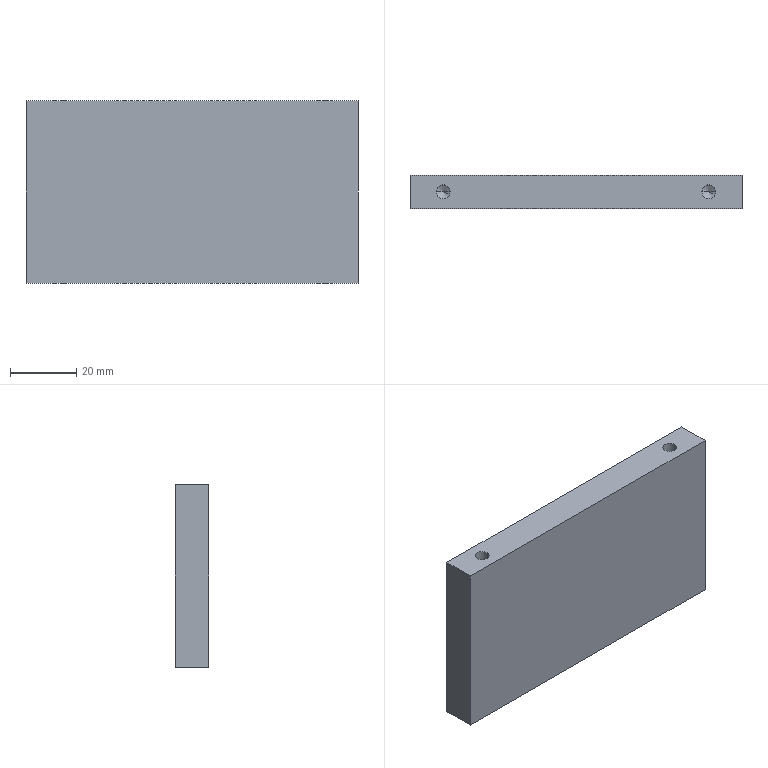Part | STEP file | PN_0036 vibratory vertical plate | 1 solid | 22 faces | box 100 x 10 x 55 mm | volume 54201 mm3 | cylinder 8 | cone 8 | plane 6 | commonest cylinder face diameters 4.2 x8
STEP:
#1=CARTESIAN_POINT('',(0.,0.,0.));
#2=DIRECTION('',(0.,0.,1.));
#3=DIRECTION('',(1.,0.,0.));
#4=AXIS2_PLACEMENT_3D('',#1,#2,#3);
#5=CARTESIAN_POINT('',(-42.1,0.,14.));
#6=VERTEX_POINT('',#5);
#7=CARTESIAN_POINT('',(-42.1,0.,0.));
#8=VERTEX_POINT('',#7);
#9=CARTESIAN_POINT('',(-42.1,0.,0.));
#10=DIRECTION('',(0.,0.,-1.));
#11=VECTOR('',#10,1.);
#12=LINE('',#9,#11);
#13=CARTESIAN_POINT('',(-40.,0.,0.));
#14=DIRECTION('',(0.,0.,-1.));
#15=DIRECTION('',(-1.,0.,0.));
#16=AXIS2_PLACEMENT_3D('',#13,#14,#15);
#17=CYLINDRICAL_SURFACE('',#16,2.1);
#18=CARTESIAN_POINT('',(6.283,0.));
#19=DIRECTION('',(0.,1.));
#20=VECTOR('',#19,1.);
#21=LINE('',#18,#20);
#22=(GEOMETRIC_REPRESENTATION_CONTEXT(2)PARAMETRIC_REPRESENTATION_CONTEXT()REPRESENTATION_CONTEXT('',''));
#23=DEFINITIONAL_REPRESENTATION('',(#21),#22);
#24=PCURVE('',#17,#23);
#25=CARTESIAN_POINT('',(-40.,0.,0.));
#26=DIRECTION('',(0.,0.,-1.));
#27=DIRECTION('',(-1.,0.,0.));
#28=AXIS2_PLACEMENT_3D('',#25,#26,#27);
#29=CYLINDRICAL_SURFACE('',#28,2.1);
#30=CARTESIAN_POINT('',(0.,0.));
#31=DIRECTION('',(0.,1.));
#32=VECTOR('',#31,1.);
#33=LINE('',#30,#32);
#34=(GEOMETRIC_REPRESENTATION_CONTEXT(2)PARAMETRIC_REPRESENTATION_CONTEXT()REPRESENTATION_CONTEXT('',''));
#35=DEFINITIONAL_REPRESENTATION('',(#33),#34);
#36=PCURVE('',#29,#35);
#37=SURFACE_CURVE('',#12,(#24,#36),.PCURVE_S1.);
#38=EDGE_CURVE('',#6,#8,#37,.T.);
#39=ORIENTED_EDGE('',*,*,#38,.T.);
#40=CARTESIAN_POINT('',(-37.9,0.,0.));
#41=VERTEX_POINT('',#40);
#42=CARTESIAN_POINT('',(-40.,0.,0.));
#43=DIRECTION('',(0.,0.,-1.));
#44=DIRECTION('',(-1.,0.,0.));
#45=AXIS2_PLACEMENT_3D('',#42,#43,#44);
#46=CIRCLE('',#45,2.1);
#47=CARTESIAN_POINT('',(0.,0.));
#48=DIRECTION('',(1.,0.));
#49=VECTOR('',#48,1.);
#50=LINE('',#47,#49);
#51=(GEOMETRIC_REPRESENTATION_CONTEXT(2)PARAMETRIC_REPRESENTATION_CONTEXT()REPRESENTATION_CONTEXT('',''));
#52=DEFINITIONAL_REPRESENTATION('',(#50),#51);
#53=PCURVE('',#17,#52);
#54=CARTESIAN_POINT('',(0.,0.,0.));
#55=DIRECTION('',(0.,0.,-1.));
#56=DIRECTION('',(-1.,0.,0.));
#57=AXIS2_PLACEMENT_3D('',#54,#55,#56);
#58=PLANE('',#57);
#59=CARTESIAN_POINT('',(40.,0.));
#60=DIRECTION('',(1.,0.));
#61=AXIS2_PLACEMENT_2D('',#59,#60);
#62=CIRCLE('',#61,2.1);
#63=(GEOMETRIC_REPRESENTATION_CONTEXT(2)PARAMETRIC_REPRESENTATION_CONTEXT()REPRESENTATION_CONTEXT('',''));
#64=DEFINITIONAL_REPRESENTATION('',(#62),#63);
#65=PCURVE('',#58,#64);
#66=SURFACE_CURVE('',#46,(#53,#65),.PCURVE_S1.);
#67=EDGE_CURVE('',#41,#8,#66,.T.);
#68=ORIENTED_EDGE('',*,*,#67,.F.);
#69=CARTESIAN_POINT('',(-37.9,0.,14.));
#70=VERTEX_POINT('',#69);
#71=CARTESIAN_POINT('',(-37.9,0.,0.));
#72=DIRECTION('',(0.,0.,-1.));
#73=VECTOR('',#72,1.);
#74=LINE('',#71,#73);
#75=CARTESIAN_POINT('',(3.142,0.));
#76=DIRECTION('',(0.,1.));
#77=VECTOR('',#76,1.);
#78=LINE('',#75,#77);
#79=(GEOMETRIC_REPRESENTATION_CONTEXT(2)PARAMETRIC_REPRESENTATION_CONTEXT()REPRESENTATION_CONTEXT('',''));
#80=DEFINITIONAL_REPRESENTATION('',(#78),#79);
#81=PCURVE('',#17,#80);
#82=CARTESIAN_POINT('',(3.142,0.));
#83=DIRECTION('',(0.,1.));
#84=VECTOR('',#83,1.);
#85=LINE('',#82,#84);
#86=(GEOMETRIC_REPRESENTATION_CONTEXT(2)PARAMETRIC_REPRESENTATION_CONTEXT()REPRESENTATION_CONTEXT('',''));
#87=DEFINITIONAL_REPRESENTATION('',(#85),#86);
#88=PCURVE('',#29,#87);
#89=SURFACE_CURVE('',#74,(#81,#88),.PCURVE_S1.);
#90=EDGE_CURVE('',#70,#41,#89,.T.);
#91=ORIENTED_EDGE('',*,*,#90,.F.);
#92=CARTESIAN_POINT('',(-40.,0.,14.));
#93=DIRECTION('',(0.,0.,-1.));
#94=DIRECTION('',(-1.,0.,0.));
#95=AXIS2_PLACEMENT_3D('',#92,#93,#94);
#96=CIRCLE('',#95,2.1);
#97=CARTESIAN_POINT('',(0.,-14.));
#98=DIRECTION('',(1.,0.));
#99=VECTOR('',#98,1.);
#100=LINE('',#97,#99);
#101=(GEOMETRIC_REPRESENTATION_CONTEXT(2)PARAMETRIC_REPRESENTATION_CONTEXT()REPRESENTATION_CONTEXT('',''));
#102=DEFINITIONAL_REPRESENTATION('',(#100),#101);
#103=PCURVE('',#17,#102);
#104=CARTESIAN_POINT('',(-40.,0.,14.));
#105=DIRECTION('',(0.,0.,-1.));
#106=DIRECTION('',(-1.,0.,0.));
#107=AXIS2_PLACEMENT_3D('',#104,#105,#106);
#108=CONICAL_SURFACE('',#107,2.1,1.03);
#109=CARTESIAN_POINT('',(0.,0.));
#110=DIRECTION('',(1.,0.));
#111=VECTOR('',#110,1.);
#112=LINE('',#109,#111);
#113=(GEOMETRIC_REPRESENTATION_CONTEXT(2)PARAMETRIC_REPRESENTATION_CONTEXT()REPRESENTATION_CONTEXT('',''));
#114=DEFINITIONAL_REPRESENTATION('',(#112),#113);
#115=PCURVE('',#108,#114);
#116=SURFACE_CURVE('',#96,(#103,#115),.PCURVE_S1.);
#117=EDGE_CURVE('',#70,#6,#116,.T.);
#118=ORIENTED_EDGE('',*,*,#117,.T.);
#119=EDGE_LOOP('',(#39,#68,#91,#118));
#120=FACE_BOUND('',#119,.F.);
#121=ADVANCED_FACE('',(#120),#17,.F.);
#122=ORIENTED_EDGE('',*,*,#117,.F.);
#123=CARTESIAN_POINT('',(-40.,0.,15.262));
#124=VERTEX_POINT('',#123);
#125=CARTESIAN_POINT('',(-37.9,0.,14.));
#126=DIRECTION('',(0.8572,0.,-0.515));
#127=VECTOR('',#126,1.);
#128=LINE('',#125,#127);
#129=CARTESIAN_POINT('',(3.142,0.));
#130=DIRECTION('',(0.,1.));
#131=VECTOR('',#130,1.);
#132=LINE('',#129,#131);
#133=(GEOMETRIC_REPRESENTATION_CONTEXT(2)PARAMETRIC_REPRESENTATION_CONTEXT()REPRESENTATION_CONTEXT('',''));
#134=DEFINITIONAL_REPRESENTATION('',(#132),#133);
#135=PCURVE('',#108,#134);
#136=CARTESIAN_POINT('',(-40.,0.,14.));
#137=DIRECTION('',(0.,0.,-1.));
#138=DIRECTION('',(-1.,0.,0.));
#139=AXIS2_PLACEMENT_3D('',#136,#137,#138);
#140=CONICAL_SURFACE('',#139,2.1,1.03);
#141=CARTESIAN_POINT('',(3.142,0.));
#142=DIRECTION('',(0.,1.));
#143=VECTOR('',#142,1.);
#144=LINE('',#141,#143);
#145=(GEOMETRIC_REPRESENTATION_CONTEXT(2)PARAMETRIC_REPRESENTATION_CONTEXT()REPRESENTATION_CONTEXT('',''));
#146=DEFINITIONAL_REPRESENTATION('',(#144),#145);
#147=PCURVE('',#140,#146);
#148=SURFACE_CURVE('',#128,(#135,#147),.PCURVE_S1.);
#149=EDGE_CURVE('',#124,#70,#148,.T.);
#150=ORIENTED_EDGE('',*,*,#149,.F.);
#151=CARTESIAN_POINT('',(-42.1,0.,14.));
#152=DIRECTION('',(-0.8572,0.,-0.515));
#153=VECTOR('',#152,1.);
#154=LINE('',#151,#153);
#155=CARTESIAN_POINT('',(6.283,0.));
#156=DIRECTION('',(0.,1.));
#157=VECTOR('',#156,1.);
#158=LINE('',#155,#157);
#159=(GEOMETRIC_REPRESENTATION_CONTEXT(2)PARAMETRIC_REPRESENTATION_CONTEXT()REPRESENTATION_CONTEXT('',''));
#160=DEFINITIONAL_REPRESENTATION('',(#158),#159);
#161=PCURVE('',#108,#160);
#162=CARTESIAN_POINT('',(0.,0.));
#163=DIRECTION('',(0.,1.));
#164=VECTOR('',#163,1.);
#165=LINE('',#162,#164);
#166=(GEOMETRIC_REPRESENTATION_CONTEXT(2)PARAMETRIC_REPRESENTATION_CONTEXT()REPRESENTATION_CONTEXT('',''));
#167=DEFINITIONAL_REPRESENTATION('',(#165),#166);
#168=PCURVE('',#140,#167);
#169=SURFACE_CURVE('',#154,(#161,#168),.PCURVE_S1.);
#170=EDGE_CURVE('',#124,#6,#169,.T.);
#171=ORIENTED_EDGE('',*,*,#170,.T.);
#172=EDGE_LOOP('',(#122,#150,#171));
#173=FACE_BOUND('',#172,.F.);
#174=ADVANCED_FACE('',(#173),#108,.F.);
#175=CARTESIAN_POINT('',(37.9,0.,14.));
#176=VERTEX_POINT('',#175);
#177=CARTESIAN_POINT('',(37.9,0.,0.));
#178=VERTEX_POINT('',#177);
#179=CARTESIAN_POINT('',(37.9,0.,0.));
#180=DIRECTION('',(0.,0.,-1.));
#181=VECTOR('',#180,1.);
#182=LINE('',#179,#181);
#183=CARTESIAN_POINT('',(40.,0.,0.));
#184=DIRECTION('',(0.,0.,-1.));
#185=DIRECTION('',(-1.,0.,0.));
#186=AXIS2_PLACEMENT_3D('',#183,#184,#185);
#187=CYLINDRICAL_SURFACE('',#186,2.1);
#188=CARTESIAN_POINT('',(6.283,0.));
#189=DIRECTION('',(0.,1.));
#190=VECTOR('',#189,1.);
#191=LINE('',#188,#190);
#192=(GEOMETRIC_REPRESENTATION_CONTEXT(2)PARAMETRIC_REPRESENTATION_CONTEXT()REPRESENTATION_CONTEXT('',''));
#193=DEFINITIONAL_REPRESENTATION('',(#191),#192);
#194=PCURVE('',#187,#193);
#195=CARTESIAN_POINT('',(40.,0.,0.));
#196=DIRECTION('',(0.,0.,-1.));
#197=DIRECTION('',(-1.,0.,0.));
#198=AXIS2_PLACEMENT_3D('',#195,#196,#197);
#199=CYLINDRICAL_SURFACE('',#198,2.1);
#200=CARTESIAN_POINT('',(0.,0.));
#201=DIRECTION('',(0.,1.));
#202=VECTOR('',#201,1.);
#203=LINE('',#200,#202);
#204=(GEOMETRIC_REPRESENTATION_CONTEXT(2)PARAMETRIC_REPRESENTATION_CONTEXT()REPRESENTATION_CONTEXT('',''));
#205=DEFINITIONAL_REPRESENTATION('',(#203),#204);
#206=PCURVE('',#199,#205);
#207=SURFACE_CURVE('',#182,(#194,#206),.PCURVE_S1.);
#208=EDGE_CURVE('',#176,#178,#207,.T.);
#209=ORIENTED_EDGE('',*,*,#208,.T.);
#210=CARTESIAN_POINT('',(42.1,0.,0.));
#211=VERTEX_POINT('',#210);
#212=CARTESIAN_POINT('',(40.,0.,0.));
#213=DIRECTION('',(0.,0.,-1.));
#214=DIRECTION('',(-1.,0.,0.));
#215=AXIS2_PLACEMENT_3D('',#212,#213,#214);
#216=CIRCLE('',#215,2.1);
#217=CARTESIAN_POINT('',(0.,0.));
#218=DIRECTION('',(1.,0.));
#219=VECTOR('',#218,1.);
#220=LINE('',#217,#219);
#221=(GEOMETRIC_REPRESENTATION_CONTEXT(2)PARAMETRIC_REPRESENTATION_CONTEXT()REPRESENTATION_CONTEXT('',''));
#222=DEFINITIONAL_REPRESENTATION('',(#220),#221);
#223=PCURVE('',#187,#222);
#224=CARTESIAN_POINT('',(-40.,0.));
#225=DIRECTION('',(1.,0.));
#226=AXIS2_PLACEMENT_2D('',#224,#225);
#227=CIRCLE('',#226,2.1);
#228=(GEOMETRIC_REPRESENTATION_CONTEXT(2)PARAMETRIC_REPRESENTATION_CONTEXT()REPRESENTATION_CONTEXT('',''));
#229=DEFINITIONAL_REPRESENTATION('',(#227),#228);
#230=PCURVE('',#58,#229);
#231=SURFACE_CURVE('',#216,(#223,#230),.PCURVE_S1.);
#232=EDGE_CURVE('',#211,#178,#231,.T.);
#233=ORIENTED_EDGE('',*,*,#232,.F.);
#234=CARTESIAN_POINT('',(42.1,0.,14.));
#235=VERTEX_POINT('',#234);
#236=CARTESIAN_POINT('',(42.1,0.,0.));
#237=DIRECTION('',(0.,0.,-1.));
#238=VECTOR('',#237,1.);
#239=LINE('',#236,#238);
#240=CARTESIAN_POINT('',(3.142,0.));
#241=DIRECTION('',(0.,1.));
#242=VECTOR('',#241,1.);
#243=LINE('',#240,#242);
#244=(GEOMETRIC_REPRESENTATION_CONTEXT(2)PARAMETRIC_REPRESENTATION_CONTEXT()REPRESENTATION_CONTEXT('',''));
#245=DEFINITIONAL_REPRESENTATION('',(#243),#244);
#246=PCURVE('',#187,#245);
#247=CARTESIAN_POINT('',(3.142,0.));
#248=DIRECTION('',(0.,1.));
#249=VECTOR('',#248,1.);
#250=LINE('',#247,#249);
#251=(GEOMETRIC_REPRESENTATION_CONTEXT(2)PARAMETRIC_REPRESENTATION_CONTEXT()REPRESENTATION_CONTEXT('',''));
#252=DEFINITIONAL_REPRESENTATION('',(#250),#251);
#253=PCURVE('',#199,#252);
#254=SURFACE_CURVE('',#239,(#246,#253),.PCURVE_S1.);
#255=EDGE_CURVE('',#235,#211,#254,.T.);
#256=ORIENTED_EDGE('',*,*,#255,.F.);
#257=CARTESIAN_POINT('',(40.,0.,14.));
#258=DIRECTION('',(0.,0.,-1.));
#259=DIRECTION('',(-1.,0.,0.));
#260=AXIS2_PLACEMENT_3D('',#257,#258,#259);
#261=CIRCLE('',#260,2.1);
#262=CARTESIAN_POINT('',(0.,-14.));
#263=DIRECTION('',(1.,0.));
#264=VECTOR('',#263,1.);
#265=LINE('',#262,#264);
#266=(GEOMETRIC_REPRESENTATION_CONTEXT(2)PARAMETRIC_REPRESENTATION_CONTEXT()REPRESENTATION_CONTEXT('',''));
#267=DEFINITIONAL_REPRESENTATION('',(#265),#266);
#268=PCURVE('',#187,#267);
#269=CARTESIAN_POINT('',(40.,0.,14.));
#270=DIRECTION('',(0.,0.,-1.));
#271=DIRECTION('',(-1.,0.,0.));
#272=AXIS2_PLACEMENT_3D('',#269,#270,#271);
#273=CONICAL_SURFACE('',#272,2.1,1.03);
#274=CARTESIAN_POINT('',(0.,0.));
#275=DIRECTION('',(1.,0.));
#276=VECTOR('',#275,1.);
#277=LINE('',#274,#276);
#278=(GEOMETRIC_REPRESENTATION_CONTEXT(2)PARAMETRIC_REPRESENTATION_CONTEXT()REPRESENTATION_CONTEXT('',''));
#279=DEFINITIONAL_REPRESENTATION('',(#277),#278);
#280=PCURVE('',#273,#279);
#281=SURFACE_CURVE('',#261,(#268,#280),.PCURVE_S1.);
#282=EDGE_CURVE('',#235,#176,#281,.T.);
#283=ORIENTED_EDGE('',*,*,#282,.T.);
#284=EDGE_LOOP('',(#209,#233,#256,#283));
#285=FACE_BOUND('',#284,.F.);
#286=ADVANCED_FACE('',(#285),#187,.F.);
#287=ORIENTED_EDGE('',*,*,#282,.F.);
#288=CARTESIAN_POINT('',(40.,0.,15.262));
#289=VERTEX_POINT('',#288);
#290=CARTESIAN_POINT('',(42.1,0.,14.));
#291=DIRECTION('',(0.8572,0.,-0.515));
#292=VECTOR('',#291,1.);
#293=LINE('',#290,#292);
#294=CARTESIAN_POINT('',(3.142,-1.262));
#295=CARTESIAN_POINT('',(3.142,-1.243));
#296=CARTESIAN_POINT('',(3.142,-1.204));
#297=CARTESIAN_POINT('',(3.142,-1.147));
#298=CARTESIAN_POINT('',(3.142,-1.09));
#299=CARTESIAN_POINT('',(3.142,-1.032));
#300=CARTESIAN_POINT('',(3.142,-0.975));
#301=CARTESIAN_POINT('',(3.142,-0.9177));
#302=CARTESIAN_POINT('',(3.142,-0.8603));
#303=CARTESIAN_POINT('',(3.142,-0.803));
#304=CARTESIAN_POINT('',(3.142,-0.7456));
#305=CARTESIAN_POINT('',(3.142,-0.6883));
#306=CARTESIAN_POINT('',(3.142,-0.6309));
#307=CARTESIAN_POINT('',(3.142,-0.5735));
#308=CARTESIAN_POINT('',(3.142,-0.5162));
#309=CARTESIAN_POINT('',(3.142,-0.4588));
#310=CARTESIAN_POINT('',(3.142,-0.4015));
#311=CARTESIAN_POINT('',(3.142,-0.3441));
#312=CARTESIAN_POINT('',(3.142,-0.2868));
#313=CARTESIAN_POINT('',(3.142,-0.2294));
#314=CARTESIAN_POINT('',(3.142,-0.1721));
#315=CARTESIAN_POINT('',(3.142,-0.1147));
#316=CARTESIAN_POINT('',(3.142,-0.05735));
#317=CARTESIAN_POINT('',(3.142,-0.01912));
#318=CARTESIAN_POINT('',(3.142,0.));
#319=B_SPLINE_CURVE_WITH_KNOTS('',3,(#294,#295,#296,#297,#298,#299,#300,#301,#302,#303,#304,#305,#306,#307,#308,#309,#310,#311,#312,#313,#314,#315,#316,#317,#318),.UNSPECIFIED.,.F.,.F.,(4,1,1,1,1,1,1,1,1,1,1,1,1,1,1,1,1,1,1,1,1,1,4),(-2.45,-2.339,-2.227,-2.116,-2.004,-1.893,-1.782,-1.67,-1.559,-1.448,-1.336,-1.225,-1.114,-1.002,-0.8909,-0.7795,-0.6682,-0.5568,-0.4454,-0.3341,-0.2227,-0.1114,0.),.UNSPECIFIED.);
#320=(GEOMETRIC_REPRESENTATION_CONTEXT(2)PARAMETRIC_REPRESENTATION_CONTEXT()REPRESENTATION_CONTEXT('',''));
#321=DEFINITIONAL_REPRESENTATION('',(#319),#320);
#322=PCURVE('',#273,#321);
#323=CARTESIAN_POINT('',(40.,0.,14.));
#324=DIRECTION('',(0.,0.,-1.));
#325=DIRECTION('',(-1.,0.,0.));
#326=AXIS2_PLACEMENT_3D('',#323,#324,#325);
#327=CONICAL_SURFACE('',#326,2.1,1.03);
#328=CARTESIAN_POINT('',(3.142,-1.262));
#329=CARTESIAN_POINT('',(3.142,-1.243));
#330=CARTESIAN_POINT('',(3.142,-1.204));
#331=CARTESIAN_POINT('',(3.142,-1.147));
#332=CARTESIAN_POINT('',(3.142,-1.09));
#333=CARTESIAN_POINT('',(3.142,-1.032));
#334=CARTESIAN_POINT('',(3.142,-0.975));
#335=CARTESIAN_POINT('',(3.142,-0.9177));
#336=CARTESIAN_POINT('',(3.142,-0.8603));
#337=CARTESIAN_POINT('',(3.142,-0.803));
#338=CARTESIAN_POINT('',(3.142,-0.7456));
#339=CARTESIAN_POINT('',(3.142,-0.6883));
#340=CARTESIAN_POINT('',(3.142,-0.6309));
#341=CARTESIAN_POINT('',(3.142,-0.5735));
#342=CARTESIAN_POINT('',(3.142,-0.5162));
#343=CARTESIAN_POINT('',(3.142,-0.4588));
#344=CARTESIAN_POINT('',(3.142,-0.4015));
#345=CARTESIAN_POINT('',(3.142,-0.3441));
#346=CARTESIAN_POINT('',(3.142,-0.2868));
#347=CARTESIAN_POINT('',(3.142,-0.2294));
#348=CARTESIAN_POINT('',(3.142,-0.1721));
#349=CARTESIAN_POINT('',(3.142,-0.1147));
#350=CARTESIAN_POINT('',(3.142,-0.05735));
#351=CARTESIAN_POINT('',(3.142,-0.01912));
#352=CARTESIAN_POINT('',(3.142,0.));
#353=B_SPLINE_CURVE_WITH_KNOTS('',3,(#328,#329,#330,#331,#332,#333,#334,#335,#336,#337,#338,#339,#340,#341,#342,#343,#344,#345,#346,#347,#348,#349,#350,#351,#352),.UNSPECIFIED.,.F.,.F.,(4,1,1,1,1,1,1,1,1,1,1,1,1,1,1,1,1,1,1,1,1,1,4),(-2.45,-2.339,-2.227,-2.116,-2.004,-1.893,-1.782,-1.67,-1.559,-1.448,-1.336,-1.225,-1.114,-1.002,-0.8909,-0.7795,-0.6682,-0.5568,-0.4454,-0.3341,-0.2227,-0.1114,0.),.UNSPECIFIED.);
#354=(GEOMETRIC_REPRESENTATION_CONTEXT(2)PARAMETRIC_REPRESENTATION_CONTEXT()REPRESENTATION_CONTEXT('',''));
#355=DEFINITIONAL_REPRESENTATION('',(#353),#354);
#356=PCURVE('',#327,#355);
#357=SURFACE_CURVE('',#293,(#322,#356),.PCURVE_S1.);
#358=EDGE_CURVE('',#289,#235,#357,.T.);
#359=ORIENTED_EDGE('',*,*,#358,.F.);
#360=CARTESIAN_POINT('',(37.9,0.,14.));
#361=DIRECTION('',(-0.8572,0.,-0.515));
#362=VECTOR('',#361,1.);
#363=LINE('',#360,#362);
#364=CARTESIAN_POINT('',(6.283,0.));
#365=DIRECTION('',(0.,1.));
#366=VECTOR('',#365,1.);
#367=LINE('',#364,#366);
#368=(GEOMETRIC_REPRESENTATION_CONTEXT(2)PARAMETRIC_REPRESENTATION_CONTEXT()REPRESENTATION_CONTEXT('',''));
#369=DEFINITIONAL_REPRESENTATION('',(#367),#368);
#370=PCURVE('',#273,#369);
#371=CARTESIAN_POINT('',(0.,0.));
#372=DIRECTION('',(0.,1.));
#373=VECTOR('',#372,1.);
#374=LINE('',#371,#373);
#375=(GEOMETRIC_REPRESENTATION_CONTEXT(2)PARAMETRIC_REPRESENTATION_CONTEXT()REPRESENTATION_CONTEXT('',''));
#376=DEFINITIONAL_REPRESENTATION('',(#374),#375);
#377=PCURVE('',#327,#376);
#378=SURFACE_CURVE('',#363,(#370,#377),.PCURVE_S1.);
#379=EDGE_CURVE('',#289,#176,#378,.T.);
#380=ORIENTED_EDGE('',*,*,#379,.T.);
#381=EDGE_LOOP('',(#287,#359,#380));
#382=FACE_BOUND('',#381,.F.);
#383=ADVANCED_FACE('',(#382),#273,.F.);
#384=CARTESIAN_POINT('',(-37.9,0.,41.));
#385=VERTEX_POINT('',#384);
#386=CARTESIAN_POINT('',(-37.9,0.,55.));
#387=VERTEX_POINT('',#386);
#388=CARTESIAN_POINT('',(-37.9,0.,55.));
#389=DIRECTION('',(0.,0.,1.));
#390=VECTOR('',#389,1.);
#391=LINE('',#388,#390);
#392=CARTESIAN_POINT('',(-40.,0.,55.));
#393=DIRECTION('',(0.,0.,1.));
#394=DIRECTION('',(1.,0.,0.));
#395=AXIS2_PLACEMENT_3D('',#392,#393,#394);
#396=CYLINDRICAL_SURFACE('',#395,2.1);
#397=CARTESIAN_POINT('',(6.283,0.));
#398=DIRECTION('',(0.,1.));
#399=VECTOR('',#398,1.);
#400=LINE('',#397,#399);
#401=(GEOMETRIC_REPRESENTATION_CONTEXT(2)PARAMETRIC_REPRESENTATION_CONTEXT()REPRESENTATION_CONTEXT('',''));
#402=DEFINITIONAL_REPRESENTATION('',(#400),#401);
#403=PCURVE('',#396,#402);
#404=CARTESIAN_POINT('',(-40.,0.,55.));
#405=DIRECTION('',(0.,0.,1.));
#406=DIRECTION('',(1.,0.,0.));
#407=AXIS2_PLACEMENT_3D('',#404,#405,#406);
#408=CYLINDRICAL_SURFACE('',#407,2.1);
#409=CARTESIAN_POINT('',(0.,0.));
#410=DIRECTION('',(0.,1.));
#411=VECTOR('',#410,1.);
#412=LINE('',#409,#411);
#413=(GEOMETRIC_REPRESENTATION_CONTEXT(2)PARAMETRIC_REPRESENTATION_CONTEXT()REPRESENTATION_CONTEXT('',''));
#414=DEFINITIONAL_REPRESENTATION('',(#412),#413);
#415=PCURVE('',#408,#414);
#416=SURFACE_CURVE('',#391,(#403,#415),.PCURVE_S1.);
#417=EDGE_CURVE('',#385,#387,#416,.T.);
#418=ORIENTED_EDGE('',*,*,#417,.T.);
#419=CARTESIAN_POINT('',(-42.1,0.,55.));
#420=VERTEX_POINT('',#419);
#421=CARTESIAN_POINT('',(-40.,0.,55.));
#422=DIRECTION('',(0.,0.,1.));
#423=DIRECTION('',(1.,0.,0.));
#424=AXIS2_PLACEMENT_3D('',#421,#422,#423);
#425=CIRCLE('',#424,2.1);
#426=CARTESIAN_POINT('',(0.,0.));
#427=DIRECTION('',(1.,0.));
#428=VECTOR('',#427,1.);
#429=LINE('',#426,#428);
#430=(GEOMETRIC_REPRESENTATION_CONTEXT(2)PARAMETRIC_REPRESENTATION_CONTEXT()REPRESENTATION_CONTEXT('',''));
#431=DEFINITIONAL_REPRESENTATION('',(#429),#430);
#432=PCURVE('',#396,#431);
#433=CARTESIAN_POINT('',(0.,0.,55.));
#434=DIRECTION('',(0.,0.,-1.));
#435=DIRECTION('',(-1.,0.,0.));
#436=AXIS2_PLACEMENT_3D('',#433,#434,#435);
#437=PLANE('',#436);
#438=CARTESIAN_POINT('',(37.9,0.));
#439=CARTESIAN_POINT('',(37.9,3.637));
#440=CARTESIAN_POINT('',(41.05,1.819));
#441=CARTESIAN_POINT('',(44.2,0.));
#442=CARTESIAN_POINT('',(41.05,-1.819));
#443=CARTESIAN_POINT('',(37.9,-3.637));
#444=CARTESIAN_POINT('',(37.9,0.));
#445=(BOUNDED_CURVE()B_SPLINE_CURVE(2,(#438,#439,#440,#441,#442,#443,#444),.UNSPECIFIED.,.T.,.F.)B_SPLINE_CURVE_WITH_KNOTS((1,2,2,2,2,1),(-2.094,0.,2.094,4.189,6.283,8.378),.UNSPECIFIED.)CURVE()GEOMETRIC_REPRESENTATION_ITEM()RATIONAL_B_SPLINE_CURVE((1.,0.5,1.,0.5,1.,0.5,1.))REPRESENTATION_ITEM(''));
#446=(GEOMETRIC_REPRESENTATION_CONTEXT(2)PARAMETRIC_REPRESENTATION_CONTEXT()REPRESENTATION_CONTEXT('',''));
#447=DEFINITIONAL_REPRESENTATION('',(#445),#446);
#448=PCURVE('',#437,#447);
#449=SURFACE_CURVE('',#425,(#432,#448),.PCURVE_S1.);
#450=EDGE_CURVE('',#420,#387,#449,.T.);
#451=ORIENTED_EDGE('',*,*,#450,.F.);
#452=CARTESIAN_POINT('',(-42.1,0.,41.));
#453=VERTEX_POINT('',#452);
#454=CARTESIAN_POINT('',(-42.1,0.,55.));
#455=DIRECTION('',(0.,0.,1.));
#456=VECTOR('',#455,1.);
#457=LINE('',#454,#456);
#458=CARTESIAN_POINT('',(3.142,0.));
#459=DIRECTION('',(0.,1.));
#460=VECTOR('',#459,1.);
#461=LINE('',#458,#460);
#462=(GEOMETRIC_REPRESENTATION_CONTEXT(2)PARAMETRIC_REPRESENTATION_CONTEXT()REPRESENTATION_CONTEXT('',''));
#463=DEFINITIONAL_REPRESENTATION('',(#461),#462);
#464=PCURVE('',#396,#463);
#465=CARTESIAN_POINT('',(3.142,0.));
#466=DIRECTION('',(0.,1.));
#467=VECTOR('',#466,1.);
#468=LINE('',#465,#467);
#469=(GEOMETRIC_REPRESENTATION_CONTEXT(2)PARAMETRIC_REPRESENTATION_CONTEXT()REPRESENTATION_CONTEXT('',''));
#470=DEFINITIONAL_REPRESENTATION('',(#468),#469);
#471=PCURVE('',#408,#470);
#472=SURFACE_CURVE('',#457,(#464,#471),.PCURVE_S1.);
#473=EDGE_CURVE('',#453,#420,#472,.T.);
#474=ORIENTED_EDGE('',*,*,#473,.F.);
#475=CARTESIAN_POINT('',(-40.,0.,41.));
#476=DIRECTION('',(0.,0.,1.));
#477=DIRECTION('',(1.,0.,0.));
#478=AXIS2_PLACEMENT_3D('',#475,#476,#477);
#479=CIRCLE('',#478,2.1);
#480=CARTESIAN_POINT('',(0.,-14.));
#481=DIRECTION('',(1.,0.));
#482=VECTOR('',#481,1.);
#483=LINE('',#480,#482);
#484=(GEOMETRIC_REPRESENTATION_CONTEXT(2)PARAMETRIC_REPRESENTATION_CONTEXT()REPRESENTATION_CONTEXT('',''));
#485=DEFINITIONAL_REPRESENTATION('',(#483),#484);
#486=PCURVE('',#396,#485);
#487=CARTESIAN_POINT('',(-40.,0.,41.));
#488=DIRECTION('',(0.,0.,1.));
#489=DIRECTION('',(1.,0.,0.));
#490=AXIS2_PLACEMENT_3D('',#487,#488,#489);
#491=CONICAL_SURFACE('',#490,2.1,1.03);
#492=CARTESIAN_POINT('',(0.,0.));
#493=DIRECTION('',(1.,0.));
#494=VECTOR('',#493,1.);
#495=LINE('',#492,#494);
#496=(GEOMETRIC_REPRESENTATION_CONTEXT(2)PARAMETRIC_REPRESENTATION_CONTEXT()REPRESENTATION_CONTEXT('',''));
#497=DEFINITIONAL_REPRESENTATION('',(#495),#496);
#498=PCURVE('',#491,#497);
#499=SURFACE_CURVE('',#479,(#486,#498),.PCURVE_S1.);
#500=EDGE_CURVE('',#453,#385,#499,.T.);
#501=ORIENTED_EDGE('',*,*,#500,.T.);
#502=EDGE_LOOP('',(#418,#451,#474,#501));
#503=FACE_BOUND('',#502,.F.);
#504=ADVANCED_FACE('',(#503),#396,.F.);
#505=ORIENTED_EDGE('',*,*,#500,.F.);
#506=CARTESIAN_POINT('',(-40.,0.,39.738));
#507=VERTEX_POINT('',#506);
#508=CARTESIAN_POINT('',(-42.1,0.,41.));
#509=DIRECTION('',(-0.8572,0.,0.515));
#510=VECTOR('',#509,1.);
#511=LINE('',#508,#510);
#512=CARTESIAN_POINT('',(3.142,0.));
#513=DIRECTION('',(0.,1.));
#514=VECTOR('',#513,1.);
#515=LINE('',#512,#514);
#516=(GEOMETRIC_REPRESENTATION_CONTEXT(2)PARAMETRIC_REPRESENTATION_CONTEXT()REPRESENTATION_CONTEXT('',''));
#517=DEFINITIONAL_REPRESENTATION('',(#515),#516);
#518=PCURVE('',#491,#517);
#519=CARTESIAN_POINT('',(-40.,0.,41.));
#520=DIRECTION('',(0.,0.,1.));
#521=DIRECTION('',(1.,0.,0.));
#522=AXIS2_PLACEMENT_3D('',#519,#520,#521);
#523=CONICAL_SURFACE('',#522,2.1,1.03);
#524=CARTESIAN_POINT('',(3.142,0.));
#525=DIRECTION('',(0.,1.));
#526=VECTOR('',#525,1.);
#527=LINE('',#524,#526);
#528=(GEOMETRIC_REPRESENTATION_CONTEXT(2)PARAMETRIC_REPRESENTATION_CONTEXT()REPRESENTATION_CONTEXT('',''));
#529=DEFINITIONAL_REPRESENTATION('',(#527),#528);
#530=PCURVE('',#523,#529);
#531=SURFACE_CURVE('',#511,(#518,#530),.PCURVE_S1.);
#532=EDGE_CURVE('',#507,#453,#531,.T.);
#533=ORIENTED_EDGE('',*,*,#532,.F.);
#534=CARTESIAN_POINT('',(-37.9,0.,41.));
#535=DIRECTION('',(0.8572,0.,0.515));
#536=VECTOR('',#535,1.);
#537=LINE('',#534,#536);
#538=CARTESIAN_POINT('',(6.283,0.));
#539=DIRECTION('',(0.,1.));
#540=VECTOR('',#539,1.);
#541=LINE('',#538,#540);
#542=(GEOMETRIC_REPRESENTATION_CONTEXT(2)PARAMETRIC_REPRESENTATION_CONTEXT()REPRESENTATION_CONTEXT('',''));
#543=DEFINITIONAL_REPRESENTATION('',(#541),#542);
#544=PCURVE('',#491,#543);
#545=CARTESIAN_POINT('',(0.,0.));
#546=DIRECTION('',(0.,1.));
#547=VECTOR('',#546,1.);
#548=LINE('',#545,#547);
#549=(GEOMETRIC_REPRESENTATION_CONTEXT(2)PARAMETRIC_REPRESENTATION_CONTEXT()REPRESENTATION_CONTEXT('',''));
#550=DEFINITIONAL_REPRESENTATION('',(#548),#549);
#551=PCURVE('',#523,#550);
#552=SURFACE_CURVE('',#537,(#544,#551),.PCURVE_S1.);
#553=EDGE_CURVE('',#507,#385,#552,.T.);
#554=ORIENTED_EDGE('',*,*,#553,.T.);
#555=EDGE_LOOP('',(#505,#533,#554));
#556=FACE_BOUND('',#555,.F.);
#557=ADVANCED_FACE('',(#556),#491,.F.);
#558=CARTESIAN_POINT('',(42.1,0.,41.));
#559=VERTEX_POINT('',#558);
#560=CARTESIAN_POINT('',(42.1,0.,55.));
#561=VERTEX_POINT('',#560);
#562=CARTESIAN_POINT('',(42.1,0.,55.));
#563=DIRECTION('',(0.,0.,1.));
#564=VECTOR('',#563,1.);
#565=LINE('',#562,#564);
#566=CARTESIAN_POINT('',(40.,0.,55.));
#567=DIRECTION('',(0.,0.,1.));
#568=DIRECTION('',(1.,0.,0.));
#569=AXIS2_PLACEMENT_3D('',#566,#567,#568);
#570=CYLINDRICAL_SURFACE('',#569,2.1);
#571=CARTESIAN_POINT('',(6.283,0.));
#572=DIRECTION('',(0.,1.));
#573=VECTOR('',#572,1.);
#574=LINE('',#571,#573);
#575=(GEOMETRIC_REPRESENTATION_CONTEXT(2)PARAMETRIC_REPRESENTATION_CONTEXT()REPRESENTATION_CONTEXT('',''));
#576=DEFINITIONAL_REPRESENTATION('',(#574),#575);
#577=PCURVE('',#570,#576);
#578=CARTESIAN_POINT('',(40.,0.,55.));
#579=DIRECTION('',(0.,0.,1.));
#580=DIRECTION('',(1.,0.,0.));
#581=AXIS2_PLACEMENT_3D('',#578,#579,#580);
#582=CYLINDRICAL_SURFACE('',#581,2.1);
#583=CARTESIAN_POINT('',(0.,0.));
#584=DIRECTION('',(0.,1.));
#585=VECTOR('',#584,1.);
#586=LINE('',#583,#585);
#587=(GEOMETRIC_REPRESENTATION_CONTEXT(2)PARAMETRIC_REPRESENTATION_CONTEXT()REPRESENTATION_CONTEXT('',''));
#588=DEFINITIONAL_REPRESENTATION('',(#586),#587);
#589=PCURVE('',#582,#588);
#590=SURFACE_CURVE('',#565,(#577,#589),.PCURVE_S1.);
#591=EDGE_CURVE('',#559,#561,#590,.T.);
#592=ORIENTED_EDGE('',*,*,#591,.T.);
#593=CARTESIAN_POINT('',(37.9,0.,55.));
#594=VERTEX_POINT('',#593);
#595=CARTESIAN_POINT('',(40.,0.,55.));
#596=DIRECTION('',(0.,0.,1.));
#597=DIRECTION('',(1.,0.,0.));
#598=AXIS2_PLACEMENT_3D('',#595,#596,#597);
#599=CIRCLE('',#598,2.1);
#600=CARTESIAN_POINT('',(0.,0.));
#601=DIRECTION('',(1.,0.));
#602=VECTOR('',#601,1.);
#603=LINE('',#600,#602);
#604=(GEOMETRIC_REPRESENTATION_CONTEXT(2)PARAMETRIC_REPRESENTATION_CONTEXT()REPRESENTATION_CONTEXT('',''));
#605=DEFINITIONAL_REPRESENTATION('',(#603),#604);
#606=PCURVE('',#570,#605);
#607=CARTESIAN_POINT('',(-42.1,0.));
#608=CARTESIAN_POINT('',(-42.1,3.637));
#609=CARTESIAN_POINT('',(-38.95,1.819));
#610=CARTESIAN_POINT('',(-35.8,0.));
#611=CARTESIAN_POINT('',(-38.95,-1.819));
#612=CARTESIAN_POINT('',(-42.1,-3.637));
#613=CARTESIAN_POINT('',(-42.1,0.));
#614=(BOUNDED_CURVE()B_SPLINE_CURVE(2,(#607,#608,#609,#610,#611,#612,#613),.UNSPECIFIED.,.T.,.F.)B_SPLINE_CURVE_WITH_KNOTS((1,2,2,2,2,1),(-2.094,0.,2.094,4.189,6.283,8.378),.UNSPECIFIED.)CURVE()GEOMETRIC_REPRESENTATION_ITEM()RATIONAL_B_SPLINE_CURVE((1.,0.5,1.,0.5,1.,0.5,1.))REPRESENTATION_ITEM(''));
#615=(GEOMETRIC_REPRESENTATION_CONTEXT(2)PARAMETRIC_REPRESENTATION_CONTEXT()REPRESENTATION_CONTEXT('',''));
#616=DEFINITIONAL_REPRESENTATION('',(#614),#615);
#617=PCURVE('',#437,#616);
#618=SURFACE_CURVE('',#599,(#606,#617),.PCURVE_S1.);
#619=EDGE_CURVE('',#594,#561,#618,.T.);
#620=ORIENTED_EDGE('',*,*,#619,.F.);
#621=CARTESIAN_POINT('',(37.9,0.,41.));
#622=VERTEX_POINT('',#621);
#623=CARTESIAN_POINT('',(37.9,0.,55.));
#624=DIRECTION('',(0.,0.,1.));
#625=VECTOR('',#624,1.);
#626=LINE('',#623,#625);
#627=CARTESIAN_POINT('',(3.142,0.));
#628=DIRECTION('',(0.,1.));
#629=VECTOR('',#628,1.);
#630=LINE('',#627,#629);
#631=(GEOMETRIC_REPRESENTATION_CONTEXT(2)PARAMETRIC_REPRESENTATION_CONTEXT()REPRESENTATION_CONTEXT('',''));
#632=DEFINITIONAL_REPRESENTATION('',(#630),#631);
#633=PCURVE('',#570,#632);
#634=CARTESIAN_POINT('',(3.142,0.));
#635=DIRECTION('',(0.,1.));
#636=VECTOR('',#635,1.);
#637=LINE('',#634,#636);
#638=(GEOMETRIC_REPRESENTATION_CONTEXT(2)PARAMETRIC_REPRESENTATION_CONTEXT()REPRESENTATION_CONTEXT('',''));
#639=DEFINITIONAL_REPRESENTATION('',(#637),#638);
#640=PCURVE('',#582,#639);
#641=SURFACE_CURVE('',#626,(#633,#640),.PCURVE_S1.);
#642=EDGE_CURVE('',#622,#594,#641,.T.);
#643=ORIENTED_EDGE('',*,*,#642,.F.);
#644=CARTESIAN_POINT('',(40.,0.,41.));
#645=DIRECTION('',(0.,0.,1.));
#646=DIRECTION('',(1.,0.,0.));
#647=AXIS2_PLACEMENT_3D('',#644,#645,#646);
#648=CIRCLE('',#647,2.1);
#649=CARTESIAN_POINT('',(0.,-14.));
#650=DIRECTION('',(1.,0.));
#651=VECTOR('',#650,1.);
#652=LINE('',#649,#651);
#653=(GEOMETRIC_REPRESENTATION_CONTEXT(2)PARAMETRIC_REPRESENTATION_CONTEXT()REPRESENTATION_CONTEXT('',''));
#654=DEFINITIONAL_REPRESENTATION('',(#652),#653);
#655=PCURVE('',#570,#654);
#656=CARTESIAN_POINT('',(40.,0.,41.));
#657=DIRECTION('',(0.,0.,1.));
#658=DIRECTION('',(1.,0.,0.));
#659=AXIS2_PLACEMENT_3D('',#656,#657,#658);
#660=CONICAL_SURFACE('',#659,2.1,1.03);
#661=CARTESIAN_POINT('',(0.,0.));
#662=DIRECTION('',(1.,0.));
#663=VECTOR('',#662,1.);
#664=LINE('',#661,#663);
#665=(GEOMETRIC_REPRESENTATION_CONTEXT(2)PARAMETRIC_REPRESENTATION_CONTEXT()REPRESENTATION_CONTEXT('',''));
#666=DEFINITIONAL_REPRESENTATION('',(#664),#665);
#667=PCURVE('',#660,#666);
#668=SURFACE_CURVE('',#648,(#655,#667),.PCURVE_S1.);
#669=EDGE_CURVE('',#622,#559,#668,.T.);
#670=ORIENTED_EDGE('',*,*,#669,.T.);
#671=EDGE_LOOP('',(#592,#620,#643,#670));
#672=FACE_BOUND('',#671,.F.);
#673=ADVANCED_FACE('',(#672),#570,.F.);
#674=ORIENTED_EDGE('',*,*,#669,.F.);
#675=CARTESIAN_POINT('',(40.,0.,39.738));
#676=VERTEX_POINT('',#675);
#677=CARTESIAN_POINT('',(37.9,0.,41.));
#678=DIRECTION('',(-0.8572,0.,0.515));
#679=VECTOR('',#678,1.);
#680=LINE('',#677,#679);
#681=CARTESIAN_POINT('',(3.142,0.));
#682=DIRECTION('',(0.,1.));
#683=VECTOR('',#682,1.);
#684=LINE('',#681,#683);
#685=(GEOMETRIC_REPRESENTATION_CONTEXT(2)PARAMETRIC_REPRESENTATION_CONTEXT()REPRESENTATION_CONTEXT('',''));
#686=DEFINITIONAL_REPRESENTATION('',(#684),#685);
#687=PCURVE('',#660,#686);
#688=CARTESIAN_POINT('',(40.,0.,41.));
#689=DIRECTION('',(0.,0.,1.));
#690=DIRECTION('',(1.,0.,0.));
#691=AXIS2_PLACEMENT_3D('',#688,#689,#690);
#692=CONICAL_SURFACE('',#691,2.1,1.03);
#693=CARTESIAN_POINT('',(3.142,0.));
#694=DIRECTION('',(0.,1.));
#695=VECTOR('',#694,1.);
#696=LINE('',#693,#695);
#697=(GEOMETRIC_REPRESENTATION_CONTEXT(2)PARAMETRIC_REPRESENTATION_CONTEXT()REPRESENTATION_CONTEXT('',''));
#698=DEFINITIONAL_REPRESENTATION('',(#696),#697);
#699=PCURVE('',#692,#698);
#700=SURFACE_CURVE('',#680,(#687,#699),.PCURVE_S1.);
#701=EDGE_CURVE('',#676,#622,#700,.T.);
#702=ORIENTED_EDGE('',*,*,#701,.F.);
#703=CARTESIAN_POINT('',(42.1,0.,41.));
#704=DIRECTION('',(0.8572,0.,0.515));
#705=VECTOR('',#704,1.);
#706=LINE('',#703,#705);
#707=CARTESIAN_POINT('',(6.283,0.));
#708=DIRECTION('',(0.,1.));
#709=VECTOR('',#708,1.);
#710=LINE('',#707,#709);
#711=(GEOMETRIC_REPRESENTATION_CONTEXT(2)PARAMETRIC_REPRESENTATION_CONTEXT()REPRESENTATION_CONTEXT('',''));
#712=DEFINITIONAL_REPRESENTATION('',(#710),#711);
#713=PCURVE('',#660,#712);
#714=CARTESIAN_POINT('',(0.,0.));
#715=DIRECTION('',(0.,1.));
#716=VECTOR('',#715,1.);
#717=LINE('',#714,#716);
#718=(GEOMETRIC_REPRESENTATION_CONTEXT(2)PARAMETRIC_REPRESENTATION_CONTEXT()REPRESENTATION_CONTEXT('',''));
#719=DEFINITIONAL_REPRESENTATION('',(#717),#718);
#720=PCURVE('',#692,#719);
#721=SURFACE_CURVE('',#706,(#713,#720),.PCURVE_S1.);
#722=EDGE_CURVE('',#676,#559,#721,.T.);
#723=ORIENTED_EDGE('',*,*,#722,.T.);
#724=EDGE_LOOP('',(#674,#702,#723));
#725=FACE_BOUND('',#724,.F.);
#726=ADVANCED_FACE('',(#725),#660,.F.);
#727=CARTESIAN_POINT('',(50.,-5.,0.));
#728=VERTEX_POINT('',#727);
#729=CARTESIAN_POINT('',(50.,5.,0.));
#730=VERTEX_POINT('',#729);
#731=CARTESIAN_POINT('',(50.,-5.,0.));
#732=DIRECTION('',(0.,1.,0.));
#733=VECTOR('',#732,1.);
#734=LINE('',#731,#733);
#735=CARTESIAN_POINT('',(50.,-5.,55.));
#736=DIRECTION('',(-1.,0.,0.));
#737=DIRECTION('',(0.,0.,1.));
#738=AXIS2_PLACEMENT_3D('',#735,#736,#737);
#739=PLANE('',#738);
#740=CARTESIAN_POINT('',(-55.,0.));
#741=DIRECTION('',(0.,1.));
#742=VECTOR('',#741,1.);
#743=LINE('',#740,#742);
#744=(GEOMETRIC_REPRESENTATION_CONTEXT(2)PARAMETRIC_REPRESENTATION_CONTEXT()REPRESENTATION_CONTEXT('',''));
#745=DEFINITIONAL_REPRESENTATION('',(#743),#744);
#746=PCURVE('',#739,#745);
#747=CARTESIAN_POINT('',(-50.,-5.));
#748=DIRECTION('',(0.,1.));
#749=VECTOR('',#748,1.);
#750=LINE('',#747,#749);
#751=(GEOMETRIC_REPRESENTATION_CONTEXT(2)PARAMETRIC_REPRESENTATION_CONTEXT()REPRESENTATION_CONTEXT('',''));
#752=DEFINITIONAL_REPRESENTATION('',(#750),#751);
#753=PCURVE('',#58,#752);
#754=SURFACE_CURVE('',#734,(#746,#753),.PCURVE_S1.);
#755=EDGE_CURVE('',#728,#730,#754,.T.);
#756=ORIENTED_EDGE('',*,*,#755,.T.);
#757=CARTESIAN_POINT('',(50.,5.,55.));
#758=VERTEX_POINT('',#757);
#759=CARTESIAN_POINT('',(50.,5.,55.));
#760=DIRECTION('',(0.,0.,-1.));
#761=VECTOR('',#760,1.);
#762=LINE('',#759,#761);
#763=CARTESIAN_POINT('',(0.,10.));
#764=DIRECTION('',(-1.,0.));
#765=VECTOR('',#764,1.);
#766=LINE('',#763,#765);
#767=(GEOMETRIC_REPRESENTATION_CONTEXT(2)PARAMETRIC_REPRESENTATION_CONTEXT()REPRESENTATION_CONTEXT('',''));
#768=DEFINITIONAL_REPRESENTATION('',(#766),#767);
#769=PCURVE('',#739,#768);
#770=CARTESIAN_POINT('',(-50.,5.,55.));
#771=DIRECTION('',(0.,-1.,0.));
#772=DIRECTION('',(0.,0.,-1.));
#773=AXIS2_PLACEMENT_3D('',#770,#771,#772);
#774=PLANE('',#773);
#775=CARTESIAN_POINT('',(0.,100.));
#776=DIRECTION('',(1.,0.));
#777=VECTOR('',#776,1.);
#778=LINE('',#775,#777);
#779=(GEOMETRIC_REPRESENTATION_CONTEXT(2)PARAMETRIC_REPRESENTATION_CONTEXT()REPRESENTATION_CONTEXT('',''));
#780=DEFINITIONAL_REPRESENTATION('',(#778),#779);
#781=PCURVE('',#774,#780);
#782=SURFACE_CURVE('',#762,(#769,#781),.PCURVE_S1.);
#783=EDGE_CURVE('',#758,#730,#782,.T.);
#784=ORIENTED_EDGE('',*,*,#783,.F.);
#785=CARTESIAN_POINT('',(50.,-5.,55.));
#786=VERTEX_POINT('',#785);
#787=CARTESIAN_POINT('',(50.,-5.,55.));
#788=DIRECTION('',(0.,1.,0.));
#789=VECTOR('',#788,1.);
#790=LINE('',#787,#789);
#791=CARTESIAN_POINT('',(0.,0.));
#792=DIRECTION('',(0.,1.));
#793=VECTOR('',#792,1.);
#794=LINE('',#791,#793);
#795=(GEOMETRIC_REPRESENTATION_CONTEXT(2)PARAMETRIC_REPRESENTATION_CONTEXT()REPRESENTATION_CONTEXT('',''));
#796=DEFINITIONAL_REPRESENTATION('',(#794),#795);
#797=PCURVE('',#739,#796);
#798=CARTESIAN_POINT('',(-50.,-5.));
#799=DIRECTION('',(0.,1.));
#800=VECTOR('',#799,1.);
#801=LINE('',#798,#800);
#802=(GEOMETRIC_REPRESENTATION_CONTEXT(2)PARAMETRIC_REPRESENTATION_CONTEXT()REPRESENTATION_CONTEXT('',''));
#803=DEFINITIONAL_REPRESENTATION('',(#801),#802);
#804=PCURVE('',#437,#803);
#805=SURFACE_CURVE('',#790,(#797,#804),.PCURVE_S1.);
#806=EDGE_CURVE('',#786,#758,#805,.T.);
#807=ORIENTED_EDGE('',*,*,#806,.F.);
#808=CARTESIAN_POINT('',(50.,-5.,55.));
#809=DIRECTION('',(0.,0.,-1.));
#810=VECTOR('',#809,1.);
#811=LINE('',#808,#810);
#812=CARTESIAN_POINT('',(0.,0.));
#813=DIRECTION('',(-1.,0.));
#814=VECTOR('',#813,1.);
#815=LINE('',#812,#814);
#816=(GEOMETRIC_REPRESENTATION_CONTEXT(2)PARAMETRIC_REPRESENTATION_CONTEXT()REPRESENTATION_CONTEXT('',''));
#817=DEFINITIONAL_REPRESENTATION('',(#815),#816);
#818=PCURVE('',#739,#817);
#819=CARTESIAN_POINT('',(-50.,-5.,55.));
#820=DIRECTION('',(0.,1.,0.));
#821=DIRECTION('',(0.,0.,1.));
#822=AXIS2_PLACEMENT_3D('',#819,#820,#821);
#823=PLANE('',#822);
#824=CARTESIAN_POINT('',(0.,100.));
#825=DIRECTION('',(-1.,0.));
#826=VECTOR('',#825,1.);
#827=LINE('',#824,#826);
#828=(GEOMETRIC_REPRESENTATION_CONTEXT(2)PARAMETRIC_REPRESENTATION_CONTEXT()REPRESENTATION_CONTEXT('',''));
#829=DEFINITIONAL_REPRESENTATION('',(#827),#828);
#830=PCURVE('',#823,#829);
#831=SURFACE_CURVE('',#811,(#818,#830),.PCURVE_S1.);
#832=EDGE_CURVE('',#786,#728,#831,.T.);
#833=ORIENTED_EDGE('',*,*,#832,.T.);
#834=EDGE_LOOP('',(#756,#784,#807,#833));
#835=FACE_BOUND('',#834,.T.);
#836=ADVANCED_FACE('',(#835),#739,.F.);
#837=CARTESIAN_POINT('',(-50.,5.,0.));
#838=VERTEX_POINT('',#837);
#839=CARTESIAN_POINT('',(-50.,5.,0.));
#840=DIRECTION('',(-1.,0.,0.));
#841=VECTOR('',#840,1.);
#842=LINE('',#839,#841);
#843=CARTESIAN_POINT('',(55.,0.));
#844=DIRECTION('',(0.,-1.));
#845=VECTOR('',#844,1.);
#846=LINE('',#843,#845);
#847=(GEOMETRIC_REPRESENTATION_CONTEXT(2)PARAMETRIC_REPRESENTATION_CONTEXT()REPRESENTATION_CONTEXT('',''));
#848=DEFINITIONAL_REPRESENTATION('',(#846),#847);
#849=PCURVE('',#774,#848);
#850=CARTESIAN_POINT('',(50.,5.));
#851=DIRECTION('',(1.,0.));
#852=VECTOR('',#851,1.);
#853=LINE('',#850,#852);
#854=(GEOMETRIC_REPRESENTATION_CONTEXT(2)PARAMETRIC_REPRESENTATION_CONTEXT()REPRESENTATION_CONTEXT('',''));
#855=DEFINITIONAL_REPRESENTATION('',(#853),#854);
#856=PCURVE('',#58,#855);
#857=SURFACE_CURVE('',#842,(#849,#856),.PCURVE_S1.);
#858=EDGE_CURVE('',#730,#838,#857,.T.);
#859=ORIENTED_EDGE('',*,*,#858,.T.);
#860=CARTESIAN_POINT('',(-50.,5.,55.));
#861=VERTEX_POINT('',#860);
#862=CARTESIAN_POINT('',(-50.,5.,55.));
#863=DIRECTION('',(0.,0.,-1.));
#864=VECTOR('',#863,1.);
#865=LINE('',#862,#864);
#866=CARTESIAN_POINT('',(0.,0.));
#867=DIRECTION('',(1.,0.));
#868=VECTOR('',#867,1.);
#869=LINE('',#866,#868);
#870=(GEOMETRIC_REPRESENTATION_CONTEXT(2)PARAMETRIC_REPRESENTATION_CONTEXT()REPRESENTATION_CONTEXT('',''));
#871=DEFINITIONAL_REPRESENTATION('',(#869),#870);
#872=PCURVE('',#774,#871);
#873=CARTESIAN_POINT('',(-50.,-5.,55.));
#874=DIRECTION('',(1.,0.,0.));
#875=DIRECTION('',(0.,0.,-1.));
#876=AXIS2_PLACEMENT_3D('',#873,#874,#875);
#877=PLANE('',#876);
#878=CARTESIAN_POINT('',(0.,10.));
#879=DIRECTION('',(1.,0.));
#880=VECTOR('',#879,1.);
#881=LINE('',#878,#880);
#882=(GEOMETRIC_REPRESENTATION_CONTEXT(2)PARAMETRIC_REPRESENTATION_CONTEXT()REPRESENTATION_CONTEXT('',''));
#883=DEFINITIONAL_REPRESENTATION('',(#881),#882);
#884=PCURVE('',#877,#883);
#885=SURFACE_CURVE('',#865,(#872,#884),.PCURVE_S1.);
#886=EDGE_CURVE('',#861,#838,#885,.T.);
#887=ORIENTED_EDGE('',*,*,#886,.F.);
#888=CARTESIAN_POINT('',(-50.,5.,55.));
#889=DIRECTION('',(-1.,0.,0.));
#890=VECTOR('',#889,1.);
#891=LINE('',#888,#890);
#892=CARTESIAN_POINT('',(0.,0.));
#893=DIRECTION('',(0.,-1.));
#894=VECTOR('',#893,1.);
#895=LINE('',#892,#894);
#896=(GEOMETRIC_REPRESENTATION_CONTEXT(2)PARAMETRIC_REPRESENTATION_CONTEXT()REPRESENTATION_CONTEXT('',''));
#897=DEFINITIONAL_REPRESENTATION('',(#895),#896);
#898=PCURVE('',#774,#897);
#899=CARTESIAN_POINT('',(50.,5.));
#900=DIRECTION('',(1.,0.));
#901=VECTOR('',#900,1.);
#902=LINE('',#899,#901);
#903=(GEOMETRIC_REPRESENTATION_CONTEXT(2)PARAMETRIC_REPRESENTATION_CONTEXT()REPRESENTATION_CONTEXT('',''));
#904=DEFINITIONAL_REPRESENTATION('',(#902),#903);
#905=PCURVE('',#437,#904);
#906=SURFACE_CURVE('',#891,(#898,#905),.PCURVE_S1.);
#907=EDGE_CURVE('',#758,#861,#906,.T.);
#908=ORIENTED_EDGE('',*,*,#907,.F.);
#909=ORIENTED_EDGE('',*,*,#783,.T.);
#910=EDGE_LOOP('',(#859,#887,#908,#909));
#911=FACE_BOUND('',#910,.T.);
#912=ADVANCED_FACE('',(#911),#774,.F.);
#913=CARTESIAN_POINT('',(-50.,-5.,0.));
#914=VERTEX_POINT('',#913);
#915=CARTESIAN_POINT('',(-50.,-5.,0.));
#916=DIRECTION('',(0.,-1.,0.));
#917=VECTOR('',#916,1.);
#918=LINE('',#915,#917);
#919=CARTESIAN_POINT('',(55.,0.));
#920=DIRECTION('',(0.,-1.));
#921=VECTOR('',#920,1.);
#922=LINE('',#919,#921);
#923=(GEOMETRIC_REPRESENTATION_CONTEXT(2)PARAMETRIC_REPRESENTATION_CONTEXT()REPRESENTATION_CONTEXT('',''));
#924=DEFINITIONAL_REPRESENTATION('',(#922),#923);
#925=PCURVE('',#877,#924);
#926=CARTESIAN_POINT('',(50.,-5.));
#927=DIRECTION('',(0.,-1.));
#928=VECTOR('',#927,1.);
#929=LINE('',#926,#928);
#930=(GEOMETRIC_REPRESENTATION_CONTEXT(2)PARAMETRIC_REPRESENTATION_CONTEXT()REPRESENTATION_CONTEXT('',''));
#931=DEFINITIONAL_REPRESENTATION('',(#929),#930);
#932=PCURVE('',#58,#931);
#933=SURFACE_CURVE('',#918,(#925,#932),.PCURVE_S1.);
#934=EDGE_CURVE('',#838,#914,#933,.T.);
#935=ORIENTED_EDGE('',*,*,#934,.T.);
#936=CARTESIAN_POINT('',(-50.,-5.,55.));
#937=VERTEX_POINT('',#936);
#938=CARTESIAN_POINT('',(-50.,-5.,55.));
#939=DIRECTION('',(0.,0.,-1.));
#940=VECTOR('',#939,1.);
#941=LINE('',#938,#940);
#942=CARTESIAN_POINT('',(0.,0.));
#943=DIRECTION('',(1.,0.));
#944=VECTOR('',#943,1.);
#945=LINE('',#942,#944);
#946=(GEOMETRIC_REPRESENTATION_CONTEXT(2)PARAMETRIC_REPRESENTATION_CONTEXT()REPRESENTATION_CONTEXT('',''));
#947=DEFINITIONAL_REPRESENTATION('',(#945),#946);
#948=PCURVE('',#877,#947);
#949=CARTESIAN_POINT('',(0.,0.));
#950=DIRECTION('',(-1.,0.));
#951=VECTOR('',#950,1.);
#952=LINE('',#949,#951);
#953=(GEOMETRIC_REPRESENTATION_CONTEXT(2)PARAMETRIC_REPRESENTATION_CONTEXT()REPRESENTATION_CONTEXT('',''));
#954=DEFINITIONAL_REPRESENTATION('',(#952),#953);
#955=PCURVE('',#823,#954);
#956=SURFACE_CURVE('',#941,(#948,#955),.PCURVE_S1.);
#957=EDGE_CURVE('',#937,#914,#956,.T.);
#958=ORIENTED_EDGE('',*,*,#957,.F.);
#959=CARTESIAN_POINT('',(-50.,-5.,55.));
#960=DIRECTION('',(0.,-1.,0.));
#961=VECTOR('',#960,1.);
#962=LINE('',#959,#961);
#963=CARTESIAN_POINT('',(0.,0.));
#964=DIRECTION('',(0.,-1.));
#965=VECTOR('',#964,1.);
#966=LINE('',#963,#965);
#967=(GEOMETRIC_REPRESENTATION_CONTEXT(2)PARAMETRIC_REPRESENTATION_CONTEXT()REPRESENTATION_CONTEXT('',''));
#968=DEFINITIONAL_REPRESENTATION('',(#966),#967);
#969=PCURVE('',#877,#968);
#970=CARTESIAN_POINT('',(50.,-5.));
#971=DIRECTION('',(0.,-1.));
#972=VECTOR('',#971,1.);
#973=LINE('',#970,#972);
#974=(GEOMETRIC_REPRESENTATION_CONTEXT(2)PARAMETRIC_REPRESENTATION_CONTEXT()REPRESENTATION_CONTEXT('',''));
#975=DEFINITIONAL_REPRESENTATION('',(#973),#974);
#976=PCURVE('',#437,#975);
#977=SURFACE_CURVE('',#962,(#969,#976),.PCURVE_S1.);
#978=EDGE_CURVE('',#861,#937,#977,.T.);
#979=ORIENTED_EDGE('',*,*,#978,.F.);
#980=ORIENTED_EDGE('',*,*,#886,.T.);
#981=EDGE_LOOP('',(#935,#958,#979,#980));
#982=FACE_BOUND('',#981,.T.);
#983=ADVANCED_FACE('',(#982),#877,.F.);
#984=CARTESIAN_POINT('',(-50.,-5.,0.));
#985=DIRECTION('',(1.,0.,0.));
#986=VECTOR('',#985,1.);
#987=LINE('',#984,#986);
#988=CARTESIAN_POINT('',(-55.,0.));
#989=DIRECTION('',(0.,1.));
#990=VECTOR('',#989,1.);
#991=LINE('',#988,#990);
#992=(GEOMETRIC_REPRESENTATION_CONTEXT(2)PARAMETRIC_REPRESENTATION_CONTEXT()REPRESENTATION_CONTEXT('',''));
#993=DEFINITIONAL_REPRESENTATION('',(#991),#992);
#994=PCURVE('',#823,#993);
#995=CARTESIAN_POINT('',(50.,-5.));
#996=DIRECTION('',(-1.,0.));
#997=VECTOR('',#996,1.);
#998=LINE('',#995,#997);
#999=(GEOMETRIC_REPRESENTATION_CONTEXT(2)PARAMETRIC_REPRESENTATION_CONTEXT()REPRESENTATION_CONTEXT('',''));
#1000=DEFINITIONAL_REPRESENTATION('',(#998),#999);
#1001=PCURVE('',#58,#1000);
#1002=SURFACE_CURVE('',#987,(#994,#1001),.PCURVE_S1.);
#1003=EDGE_CURVE('',#914,#728,#1002,.T.);
#1004=ORIENTED_EDGE('',*,*,#1003,.T.);
#1005=ORIENTED_EDGE('',*,*,#832,.F.);
#1006=CARTESIAN_POINT('',(-50.,-5.,55.));
#1007=DIRECTION('',(1.,0.,0.));
#1008=VECTOR('',#1007,1.);
#1009=LINE('',#1006,#1008);
#1010=CARTESIAN_POINT('',(0.,0.));
#1011=DIRECTION('',(0.,1.));
#1012=VECTOR('',#1011,1.);
#1013=LINE('',#1010,#1012);
#1014=(GEOMETRIC_REPRESENTATION_CONTEXT(2)PARAMETRIC_REPRESENTATION_CONTEXT()REPRESENTATION_CONTEXT('',''));
#1015=DEFINITIONAL_REPRESENTATION('',(#1013),#1014);
#1016=PCURVE('',#823,#1015);
#1017=CARTESIAN_POINT('',(50.,-5.));
#1018=DIRECTION('',(-1.,0.));
#1019=VECTOR('',#1018,1.);
#1020=LINE('',#1017,#1019);
#1021=(GEOMETRIC_REPRESENTATION_CONTEXT(2)PARAMETRIC_REPRESENTATION_CONTEXT()REPRESENTATION_CONTEXT('',''));
#1022=DEFINITIONAL_REPRESENTATION('',(#1020),#1021);
#1023=PCURVE('',#437,#1022);
#1024=SURFACE_CURVE('',#1009,(#1016,#1023),.PCURVE_S1.);
#1025=EDGE_CURVE('',#937,#786,#1024,.T.);
#1026=ORIENTED_EDGE('',*,*,#1025,.F.);
#1027=ORIENTED_EDGE('',*,*,#957,.T.);
#1028=EDGE_LOOP('',(#1004,#1005,#1026,#1027));
#1029=FACE_BOUND('',#1028,.T.);
#1030=ADVANCED_FACE('',(#1029),#823,.F.);
#1031=CARTESIAN_POINT('',(-40.,0.,55.));
#1032=DIRECTION('',(0.,0.,1.));
#1033=DIRECTION('',(1.,0.,0.));
#1034=AXIS2_PLACEMENT_3D('',#1031,#1032,#1033);
#1035=CIRCLE('',#1034,2.1);
#1036=CARTESIAN_POINT('',(37.9,0.));
#1037=CARTESIAN_POINT('',(37.9,3.637));
#1038=CARTESIAN_POINT('',(41.05,1.819));
#1039=CARTESIAN_POINT('',(44.2,0.));
#1040=CARTESIAN_POINT('',(41.05,-1.819));
#1041=CARTESIAN_POINT('',(37.9,-3.637));
#1042=CARTESIAN_POINT('',(37.9,0.));
#1043=(BOUNDED_CURVE()B_SPLINE_CURVE(2,(#1036,#1037,#1038,#1039,#1040,#1041,#1042),.UNSPECIFIED.,.T.,.F.)B_SPLINE_CURVE_WITH_KNOTS((1,2,2,2,2,1),(-2.094,0.,2.094,4.189,6.283,8.378),.UNSPECIFIED.)CURVE()GEOMETRIC_REPRESENTATION_ITEM()RATIONAL_B_SPLINE_CURVE((1.,0.5,1.,0.5,1.,0.5,1.))REPRESENTATION_ITEM(''));
#1044=(GEOMETRIC_REPRESENTATION_CONTEXT(2)PARAMETRIC_REPRESENTATION_CONTEXT()REPRESENTATION_CONTEXT('',''));
#1045=DEFINITIONAL_REPRESENTATION('',(#1043),#1044);
#1046=PCURVE('',#437,#1045);
#1047=CARTESIAN_POINT('',(0.,0.));
#1048=DIRECTION('',(1.,0.));
#1049=VECTOR('',#1048,1.);
#1050=LINE('',#1047,#1049);
#1051=(GEOMETRIC_REPRESENTATION_CONTEXT(2)PARAMETRIC_REPRESENTATION_CONTEXT()REPRESENTATION_CONTEXT('',''));
#1052=DEFINITIONAL_REPRESENTATION('',(#1050),#1051);
#1053=PCURVE('',#408,#1052);
#1054=SURFACE_CURVE('',#1035,(#1046,#1053),.PCURVE_S1.);
#1055=EDGE_CURVE('',#387,#420,#1054,.T.);
#1056=ORIENTED_EDGE('',*,*,#1055,.F.);
#1057=ORIENTED_EDGE('',*,*,#450,.F.);
#1058=EDGE_LOOP('',(#1056,#1057));
#1059=FACE_BOUND('',#1058,.T.);
#1060=CARTESIAN_POINT('',(40.,0.,55.));
#1061=DIRECTION('',(0.,0.,1.));
#1062=DIRECTION('',(1.,0.,0.));
#1063=AXIS2_PLACEMENT_3D('',#1060,#1061,#1062);
#1064=CIRCLE('',#1063,2.1);
#1065=CARTESIAN_POINT('',(-42.1,0.));
#1066=CARTESIAN_POINT('',(-42.1,3.637));
#1067=CARTESIAN_POINT('',(-38.95,1.819));
#1068=CARTESIAN_POINT('',(-35.8,0.));
#1069=CARTESIAN_POINT('',(-38.95,-1.819));
#1070=CARTESIAN_POINT('',(-42.1,-3.637));
#1071=CARTESIAN_POINT('',(-42.1,0.));
#1072=(BOUNDED_CURVE()B_SPLINE_CURVE(2,(#1065,#1066,#1067,#1068,#1069,#1070,#1071),.UNSPECIFIED.,.T.,.F.)B_SPLINE_CURVE_WITH_KNOTS((1,2,2,2,2,1),(-2.094,0.,2.094,4.189,6.283,8.378),.UNSPECIFIED.)CURVE()GEOMETRIC_REPRESENTATION_ITEM()RATIONAL_B_SPLINE_CURVE((1.,0.5,1.,0.5,1.,0.5,1.))REPRESENTATION_ITEM(''));
#1073=(GEOMETRIC_REPRESENTATION_CONTEXT(2)PARAMETRIC_REPRESENTATION_CONTEXT()REPRESENTATION_CONTEXT('',''));
#1074=DEFINITIONAL_REPRESENTATION('',(#1072),#1073);
#1075=PCURVE('',#437,#1074);
#1076=CARTESIAN_POINT('',(0.,0.));
#1077=DIRECTION('',(1.,0.));
#1078=VECTOR('',#1077,1.);
#1079=LINE('',#1076,#1078);
#1080=(GEOMETRIC_REPRESENTATION_CONTEXT(2)PARAMETRIC_REPRESENTATION_CONTEXT()REPRESENTATION_CONTEXT('',''));
#1081=DEFINITIONAL_REPRESENTATION('',(#1079),#1080);
#1082=PCURVE('',#582,#1081);
#1083=SURFACE_CURVE('',#1064,(#1075,#1082),.PCURVE_S1.);
#1084=EDGE_CURVE('',#561,#594,#1083,.T.);
#1085=ORIENTED_EDGE('',*,*,#1084,.F.);
#1086=ORIENTED_EDGE('',*,*,#619,.F.);
#1087=EDGE_LOOP('',(#1085,#1086));
#1088=FACE_BOUND('',#1087,.T.);
#1089=ORIENTED_EDGE('',*,*,#806,.T.);
#1090=ORIENTED_EDGE('',*,*,#907,.T.);
#1091=ORIENTED_EDGE('',*,*,#978,.T.);
#1092=ORIENTED_EDGE('',*,*,#1025,.T.);
#1093=EDGE_LOOP('',(#1089,#1090,#1091,#1092));
#1094=FACE_BOUND('',#1093,.T.);
#1095=ADVANCED_FACE('',(#1059,#1088,#1094),#437,.F.);
#1096=CARTESIAN_POINT('',(-40.,0.,0.));
#1097=DIRECTION('',(0.,0.,-1.));
#1098=DIRECTION('',(-1.,0.,0.));
#1099=AXIS2_PLACEMENT_3D('',#1096,#1097,#1098);
#1100=CIRCLE('',#1099,2.1);
#1101=CARTESIAN_POINT('',(40.,0.));
#1102=DIRECTION('',(1.,0.));
#1103=AXIS2_PLACEMENT_2D('',#1101,#1102);
#1104=CIRCLE('',#1103,2.1);
#1105=(GEOMETRIC_REPRESENTATION_CONTEXT(2)PARAMETRIC_REPRESENTATION_CONTEXT()REPRESENTATION_CONTEXT('',''));
#1106=DEFINITIONAL_REPRESENTATION('',(#1104),#1105);
#1107=PCURVE('',#58,#1106);
#1108=CARTESIAN_POINT('',(0.,0.));
#1109=DIRECTION('',(1.,0.));
#1110=VECTOR('',#1109,1.);
#1111=LINE('',#1108,#1110);
#1112=(GEOMETRIC_REPRESENTATION_CONTEXT(2)PARAMETRIC_REPRESENTATION_CONTEXT()REPRESENTATION_CONTEXT('',''));
#1113=DEFINITIONAL_REPRESENTATION('',(#1111),#1112);
#1114=PCURVE('',#29,#1113);
#1115=SURFACE_CURVE('',#1100,(#1107,#1114),.PCURVE_S1.);
#1116=EDGE_CURVE('',#8,#41,#1115,.T.);
#1117=ORIENTED_EDGE('',*,*,#1116,.F.);
#1118=ORIENTED_EDGE('',*,*,#67,.F.);
#1119=EDGE_LOOP('',(#1117,#1118));
#1120=FACE_BOUND('',#1119,.T.);
#1121=CARTESIAN_POINT('',(40.,0.,0.));
#1122=DIRECTION('',(0.,0.,-1.));
#1123=DIRECTION('',(-1.,0.,0.));
#1124=AXIS2_PLACEMENT_3D('',#1121,#1122,#1123);
#1125=CIRCLE('',#1124,2.1);
#1126=CARTESIAN_POINT('',(-40.,0.));
#1127=DIRECTION('',(1.,0.));
#1128=AXIS2_PLACEMENT_2D('',#1126,#1127);
#1129=CIRCLE('',#1128,2.1);
#1130=(GEOMETRIC_REPRESENTATION_CONTEXT(2)PARAMETRIC_REPRESENTATION_CONTEXT()REPRESENTATION_CONTEXT('',''));
#1131=DEFINITIONAL_REPRESENTATION('',(#1129),#1130);
#1132=PCURVE('',#58,#1131);
#1133=CARTESIAN_POINT('',(0.,0.));
#1134=DIRECTION('',(1.,0.));
#1135=VECTOR('',#1134,1.);
#1136=LINE('',#1133,#1135);
#1137=(GEOMETRIC_REPRESENTATION_CONTEXT(2)PARAMETRIC_REPRESENTATION_CONTEXT()REPRESENTATION_CONTEXT('',''));
#1138=DEFINITIONAL_REPRESENTATION('',(#1136),#1137);
#1139=PCURVE('',#199,#1138);
#1140=SURFACE_CURVE('',#1125,(#1132,#1139),.PCURVE_S1.);
#1141=EDGE_CURVE('',#178,#211,#1140,.T.);
#1142=ORIENTED_EDGE('',*,*,#1141,.F.);
#1143=ORIENTED_EDGE('',*,*,#232,.F.);
#1144=EDGE_LOOP('',(#1142,#1143));
#1145=FACE_BOUND('',#1144,.T.);
#1146=ORIENTED_EDGE('',*,*,#755,.F.);
#1147=ORIENTED_EDGE('',*,*,#1003,.F.);
#1148=ORIENTED_EDGE('',*,*,#934,.F.);
#1149=ORIENTED_EDGE('',*,*,#858,.F.);
#1150=EDGE_LOOP('',(#1146,#1147,#1148,#1149));
#1151=FACE_BOUND('',#1150,.T.);
#1152=ADVANCED_FACE('',(#1120,#1145,#1151),#58,.T.);
#1153=CARTESIAN_POINT('',(40.,0.,41.));
#1154=DIRECTION('',(0.,0.,1.));
#1155=DIRECTION('',(1.,0.,0.));
#1156=AXIS2_PLACEMENT_3D('',#1153,#1154,#1155);
#1157=CIRCLE('',#1156,2.1);
#1158=CARTESIAN_POINT('',(0.,0.));
#1159=DIRECTION('',(1.,0.));
#1160=VECTOR('',#1159,1.);
#1161=LINE('',#1158,#1160);
#1162=(GEOMETRIC_REPRESENTATION_CONTEXT(2)PARAMETRIC_REPRESENTATION_CONTEXT()REPRESENTATION_CONTEXT('',''));
#1163=DEFINITIONAL_REPRESENTATION('',(#1161),#1162);
#1164=PCURVE('',#692,#1163);
#1165=CARTESIAN_POINT('',(0.,-14.));
#1166=DIRECTION('',(1.,0.));
#1167=VECTOR('',#1166,1.);
#1168=LINE('',#1165,#1167);
#1169=(GEOMETRIC_REPRESENTATION_CONTEXT(2)PARAMETRIC_REPRESENTATION_CONTEXT()REPRESENTATION_CONTEXT('',''));
#1170=DEFINITIONAL_REPRESENTATION('',(#1168),#1169);
#1171=PCURVE('',#582,#1170);
#1172=SURFACE_CURVE('',#1157,(#1164,#1171),.PCURVE_S1.);
#1173=EDGE_CURVE('',#559,#622,#1172,.T.);
#1174=ORIENTED_EDGE('',*,*,#1173,.F.);
#1175=ORIENTED_EDGE('',*,*,#722,.F.);
#1176=ORIENTED_EDGE('',*,*,#701,.T.);
#1177=EDGE_LOOP('',(#1174,#1175,#1176));
#1178=FACE_BOUND('',#1177,.F.);
#1179=ADVANCED_FACE('',(#1178),#692,.F.);
#1180=ORIENTED_EDGE('',*,*,#1084,.F.);
#1181=ORIENTED_EDGE('',*,*,#591,.F.);
#1182=ORIENTED_EDGE('',*,*,#1173,.T.);
#1183=ORIENTED_EDGE('',*,*,#642,.T.);
#1184=EDGE_LOOP('',(#1180,#1181,#1182,#1183));
#1185=FACE_BOUND('',#1184,.F.);
#1186=ADVANCED_FACE('',(#1185),#582,.F.);
#1187=CARTESIAN_POINT('',(-40.,0.,41.));
#1188=DIRECTION('',(0.,0.,1.));
#1189=DIRECTION('',(1.,0.,0.));
#1190=AXIS2_PLACEMENT_3D('',#1187,#1188,#1189);
#1191=CIRCLE('',#1190,2.1);
#1192=CARTESIAN_POINT('',(0.,0.));
#1193=DIRECTION('',(1.,0.));
#1194=VECTOR('',#1193,1.);
#1195=LINE('',#1192,#1194);
#1196=(GEOMETRIC_REPRESENTATION_CONTEXT(2)PARAMETRIC_REPRESENTATION_CONTEXT()REPRESENTATION_CONTEXT('',''));
#1197=DEFINITIONAL_REPRESENTATION('',(#1195),#1196);
#1198=PCURVE('',#523,#1197);
#1199=CARTESIAN_POINT('',(0.,-14.));
#1200=DIRECTION('',(1.,0.));
#1201=VECTOR('',#1200,1.);
#1202=LINE('',#1199,#1201);
#1203=(GEOMETRIC_REPRESENTATION_CONTEXT(2)PARAMETRIC_REPRESENTATION_CONTEXT()REPRESENTATION_CONTEXT('',''));
#1204=DEFINITIONAL_REPRESENTATION('',(#1202),#1203);
#1205=PCURVE('',#408,#1204);
#1206=SURFACE_CURVE('',#1191,(#1198,#1205),.PCURVE_S1.);
#1207=EDGE_CURVE('',#385,#453,#1206,.T.);
#1208=ORIENTED_EDGE('',*,*,#1207,.F.);
#1209=ORIENTED_EDGE('',*,*,#553,.F.);
#1210=ORIENTED_EDGE('',*,*,#532,.T.);
#1211=EDGE_LOOP('',(#1208,#1209,#1210));
#1212=FACE_BOUND('',#1211,.F.);
#1213=ADVANCED_FACE('',(#1212),#523,.F.);
#1214=ORIENTED_EDGE('',*,*,#1055,.F.);
#1215=ORIENTED_EDGE('',*,*,#417,.F.);
#1216=ORIENTED_EDGE('',*,*,#1207,.T.);
#1217=ORIENTED_EDGE('',*,*,#473,.T.);
#1218=EDGE_LOOP('',(#1214,#1215,#1216,#1217));
#1219=FACE_BOUND('',#1218,.F.);
#1220=ADVANCED_FACE('',(#1219),#408,.F.);
#1221=CARTESIAN_POINT('',(40.,0.,14.));
#1222=DIRECTION('',(0.,0.,-1.));
#1223=DIRECTION('',(-1.,0.,0.));
#1224=AXIS2_PLACEMENT_3D('',#1221,#1222,#1223);
#1225=CIRCLE('',#1224,2.1);
#1226=CARTESIAN_POINT('',(0.,0.));
#1227=DIRECTION('',(1.,0.));
#1228=VECTOR('',#1227,1.);
#1229=LINE('',#1226,#1228);
#1230=(GEOMETRIC_REPRESENTATION_CONTEXT(2)PARAMETRIC_REPRESENTATION_CONTEXT()REPRESENTATION_CONTEXT('',''));
#1231=DEFINITIONAL_REPRESENTATION('',(#1229),#1230);
#1232=PCURVE('',#327,#1231);
#1233=CARTESIAN_POINT('',(0.,-14.));
#1234=DIRECTION('',(1.,0.));
#1235=VECTOR('',#1234,1.);
#1236=LINE('',#1233,#1235);
#1237=(GEOMETRIC_REPRESENTATION_CONTEXT(2)PARAMETRIC_REPRESENTATION_CONTEXT()REPRESENTATION_CONTEXT('',''));
#1238=DEFINITIONAL_REPRESENTATION('',(#1236),#1237);
#1239=PCURVE('',#199,#1238);
#1240=SURFACE_CURVE('',#1225,(#1232,#1239),.PCURVE_S1.);
#1241=EDGE_CURVE('',#176,#235,#1240,.T.);
#1242=ORIENTED_EDGE('',*,*,#1241,.F.);
#1243=ORIENTED_EDGE('',*,*,#379,.F.);
#1244=ORIENTED_EDGE('',*,*,#358,.T.);
#1245=EDGE_LOOP('',(#1242,#1243,#1244));
#1246=FACE_BOUND('',#1245,.F.);
#1247=ADVANCED_FACE('',(#1246),#327,.F.);
#1248=ORIENTED_EDGE('',*,*,#1141,.F.);
#1249=ORIENTED_EDGE('',*,*,#208,.F.);
#1250=ORIENTED_EDGE('',*,*,#1241,.T.);
#1251=ORIENTED_EDGE('',*,*,#255,.T.);
#1252=EDGE_LOOP('',(#1248,#1249,#1250,#1251));
#1253=FACE_BOUND('',#1252,.F.);
#1254=ADVANCED_FACE('',(#1253),#199,.F.);
#1255=CARTESIAN_POINT('',(-40.,0.,14.));
#1256=DIRECTION('',(0.,0.,-1.));
#1257=DIRECTION('',(-1.,0.,0.));
#1258=AXIS2_PLACEMENT_3D('',#1255,#1256,#1257);
#1259=CIRCLE('',#1258,2.1);
#1260=CARTESIAN_POINT('',(0.,0.));
#1261=DIRECTION('',(1.,0.));
#1262=VECTOR('',#1261,1.);
#1263=LINE('',#1260,#1262);
#1264=(GEOMETRIC_REPRESENTATION_CONTEXT(2)PARAMETRIC_REPRESENTATION_CONTEXT()REPRESENTATION_CONTEXT('',''));
#1265=DEFINITIONAL_REPRESENTATION('',(#1263),#1264);
#1266=PCURVE('',#140,#1265);
#1267=CARTESIAN_POINT('',(0.,-14.));
#1268=DIRECTION('',(1.,0.));
#1269=VECTOR('',#1268,1.);
#1270=LINE('',#1267,#1269);
#1271=(GEOMETRIC_REPRESENTATION_CONTEXT(2)PARAMETRIC_REPRESENTATION_CONTEXT()REPRESENTATION_CONTEXT('',''));
#1272=DEFINITIONAL_REPRESENTATION('',(#1270),#1271);
#1273=PCURVE('',#29,#1272);
#1274=SURFACE_CURVE('',#1259,(#1266,#1273),.PCURVE_S1.);
#1275=EDGE_CURVE('',#6,#70,#1274,.T.);
#1276=ORIENTED_EDGE('',*,*,#1275,.F.);
#1277=ORIENTED_EDGE('',*,*,#170,.F.);
#1278=ORIENTED_EDGE('',*,*,#149,.T.);
#1279=EDGE_LOOP('',(#1276,#1277,#1278));
#1280=FACE_BOUND('',#1279,.F.);
#1281=ADVANCED_FACE('',(#1280),#140,.F.);
#1282=ORIENTED_EDGE('',*,*,#1116,.F.);
#1283=ORIENTED_EDGE('',*,*,#38,.F.);
#1284=ORIENTED_EDGE('',*,*,#1275,.T.);
#1285=ORIENTED_EDGE('',*,*,#90,.T.);
#1286=EDGE_LOOP('',(#1282,#1283,#1284,#1285));
#1287=FACE_BOUND('',#1286,.F.);
#1288=ADVANCED_FACE('',(#1287),#29,.F.);
#1289=CLOSED_SHELL('',(#121,#174,#286,#383,#504,#557,#673,#726,#836,#912,#983,#1030,#1095,#1152,#1179,#1186,#1213,#1220,#1247,#1254,#1281,#1288));
#1290=MANIFOLD_SOLID_BREP('',#1289);
#1291=(LENGTH_UNIT()NAMED_UNIT(*)SI_UNIT(.MILLI.,.METRE.));
#1292=UNCERTAINTY_MEASURE_WITH_UNIT(LENGTH_MEASURE(0.0000001),#1291,'','');
#1293=(NAMED_UNIT(*)PLANE_ANGLE_UNIT()SI_UNIT($,.RADIAN.));
#1294=(NAMED_UNIT(*)SI_UNIT($,.STERADIAN.)SOLID_ANGLE_UNIT());
#1295=(GEOMETRIC_REPRESENTATION_CONTEXT(3)GLOBAL_UNCERTAINTY_ASSIGNED_CONTEXT((#1292))GLOBAL_UNIT_ASSIGNED_CONTEXT((#1291,#1293,#1294))REPRESENTATION_CONTEXT('',''));
#1296=ADVANCED_BREP_SHAPE_REPRESENTATION('',(#4,#1290),#1295);